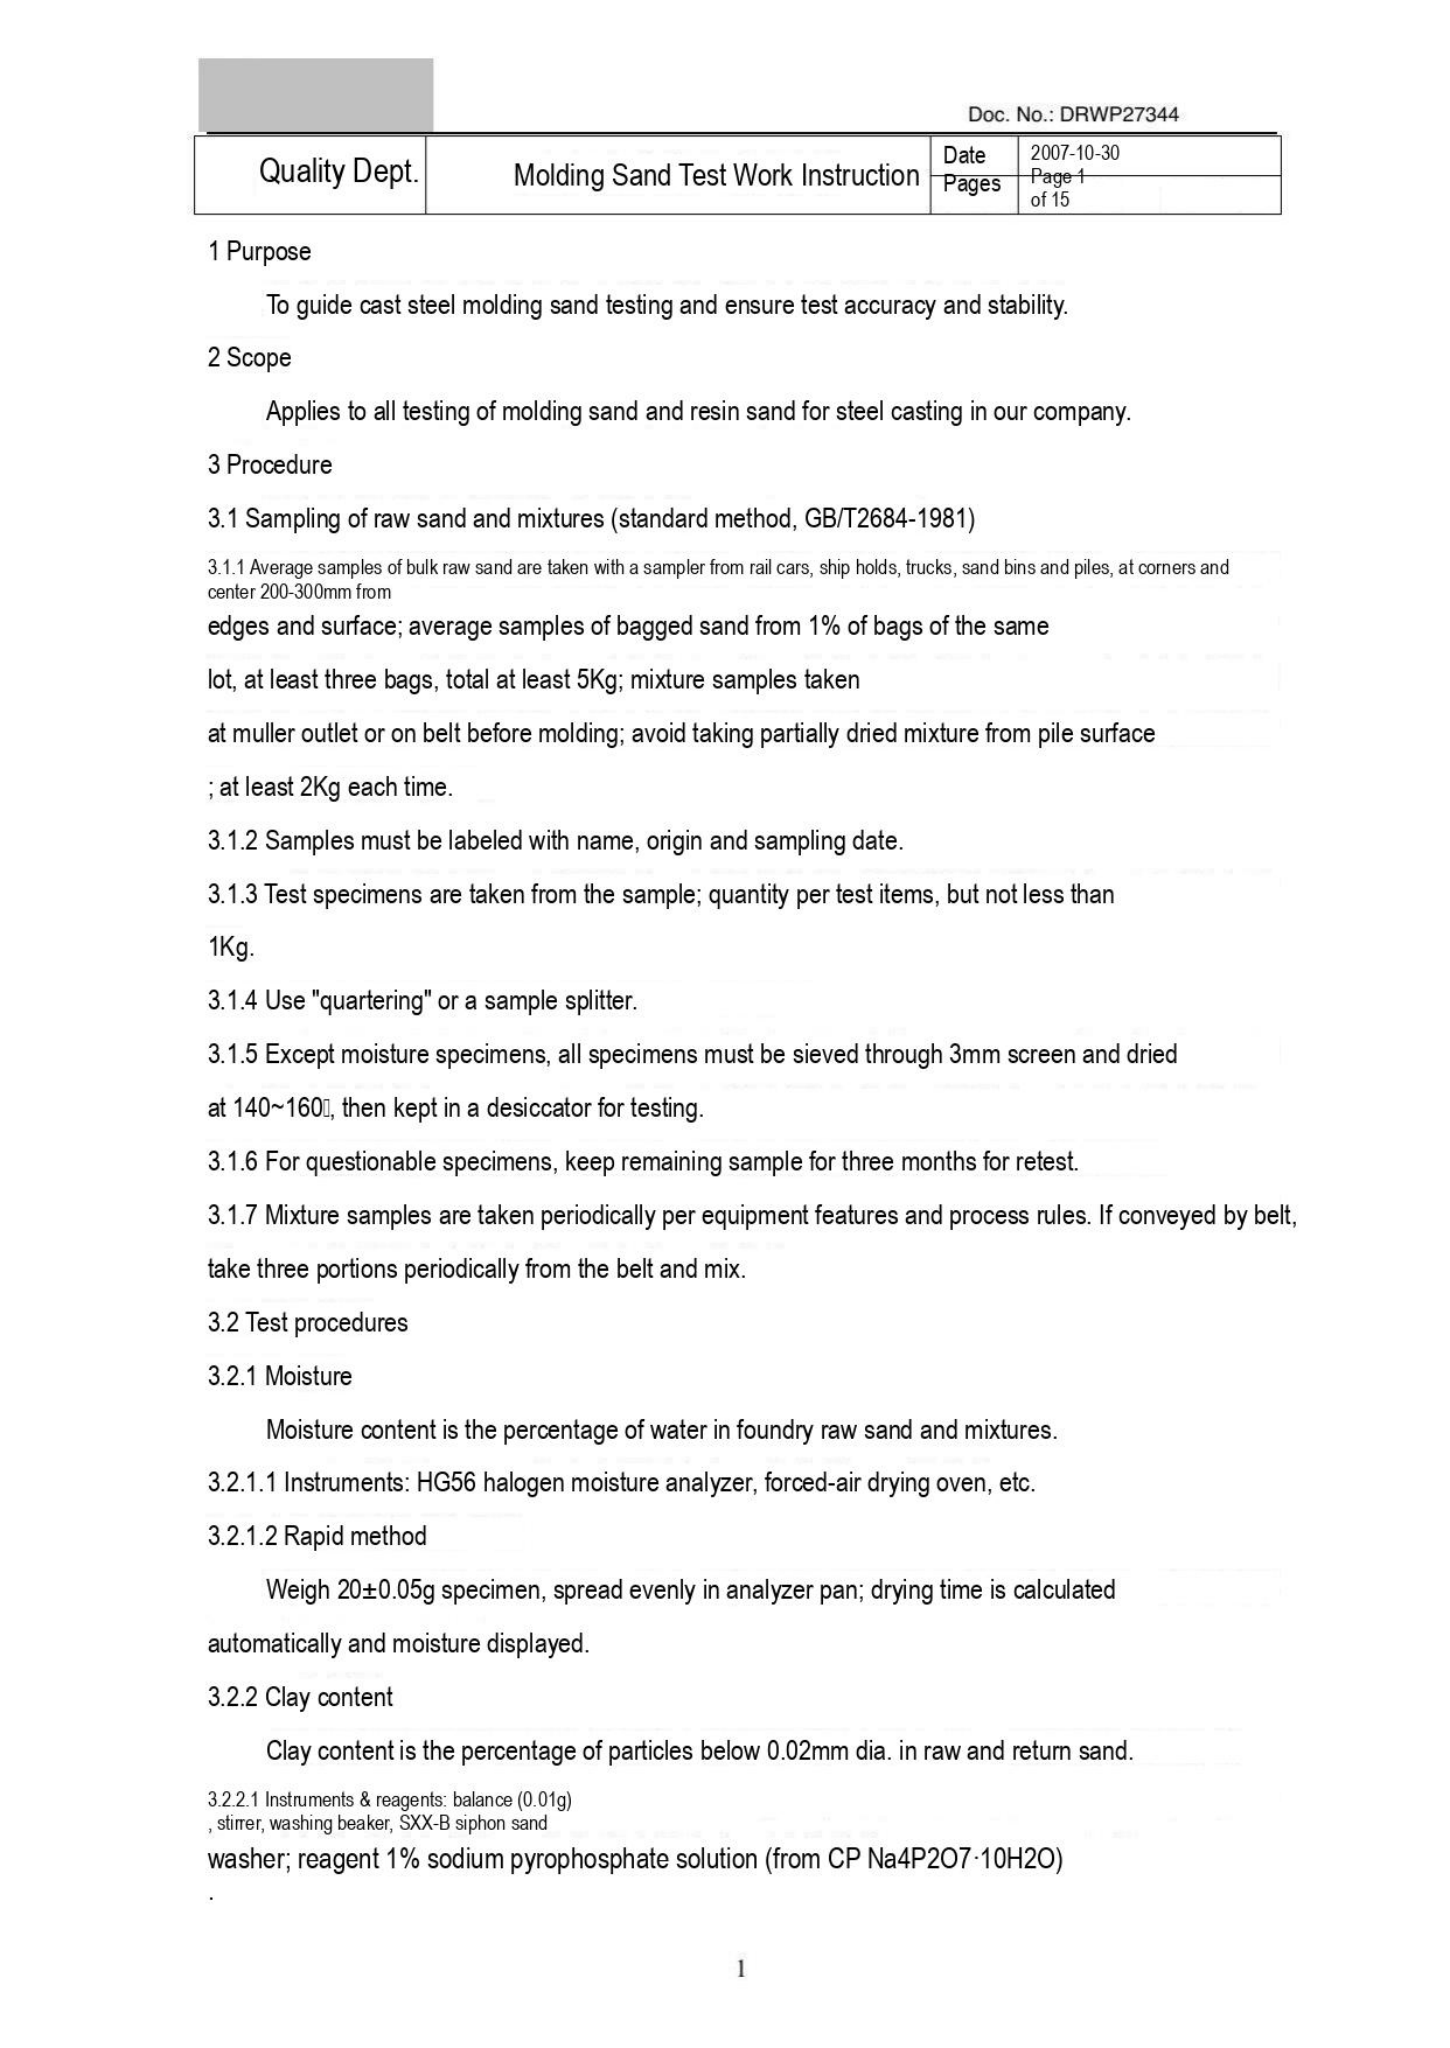Doc. No.: DRWP27344

| Quality Dept. | Molding Sand Test Work Instruction | Date | 2007-10-30 |
|---|---|---|---|
| | | Pages | Page 1 of 15 |

1 Purpose

To guide cast steel molding sand testing and ensure test accuracy and stability.

2 Scope

Applies to all testing of molding sand and resin sand for steel casting in our company.

3 Procedure

3.1 Sampling of raw sand and mixtures (standard method, GB/T2684-1981)

3.1.1 Average samples of bulk raw sand are taken with a sampler from rail cars, ship holds, trucks, sand bins and piles, at corners and center 200-300mm from edges and surface; average samples of bagged sand from 1% of bags of the same lot, at least three bags, total at least 5Kg; mixture samples taken at muller outlet or on belt before molding; avoid taking partially dried mixture from pile surface; at least 2Kg each time.

3.1.2 Samples must be labeled with name, origin and sampling date.

3.1.3 Test specimens are taken from the sample; quantity per test items, but not less than 1Kg.

3.1.4 Use "quartering" or a sample splitter.

3.1.5 Except moisture specimens, all specimens must be sieved through 3mm screen and dried at 140~160, then kept in a desiccator for testing.

3.1.6 For questionable specimens, keep remaining sample for three months for retest.

3.1.7 Mixture samples are taken periodically per equipment features and process rules. If conveyed by belt, take three portions periodically from the belt and mix.

3.2 Test procedures

3.2.1 Moisture

Moisture content is the percentage of water in foundry raw sand and mixtures.

3.2.1.1 Instruments: HG56 halogen moisture analyzer, forced-air drying oven, etc.

3.2.1.2 Rapid method

Weigh 20±0.05g specimen, spread evenly in analyzer pan; drying time is calculated automatically and moisture displayed.

3.2.2 Clay content

Clay content is the percentage of particles below 0.02mm dia. in raw and return sand.

3.2.2.1 Instruments & reagents: balance (0.01g), stirrer, washing beaker, SXX-B siphon sand washer; reagent 1% sodium pyrophosphate solution (from CP Na4P2O7·10H2O).

1
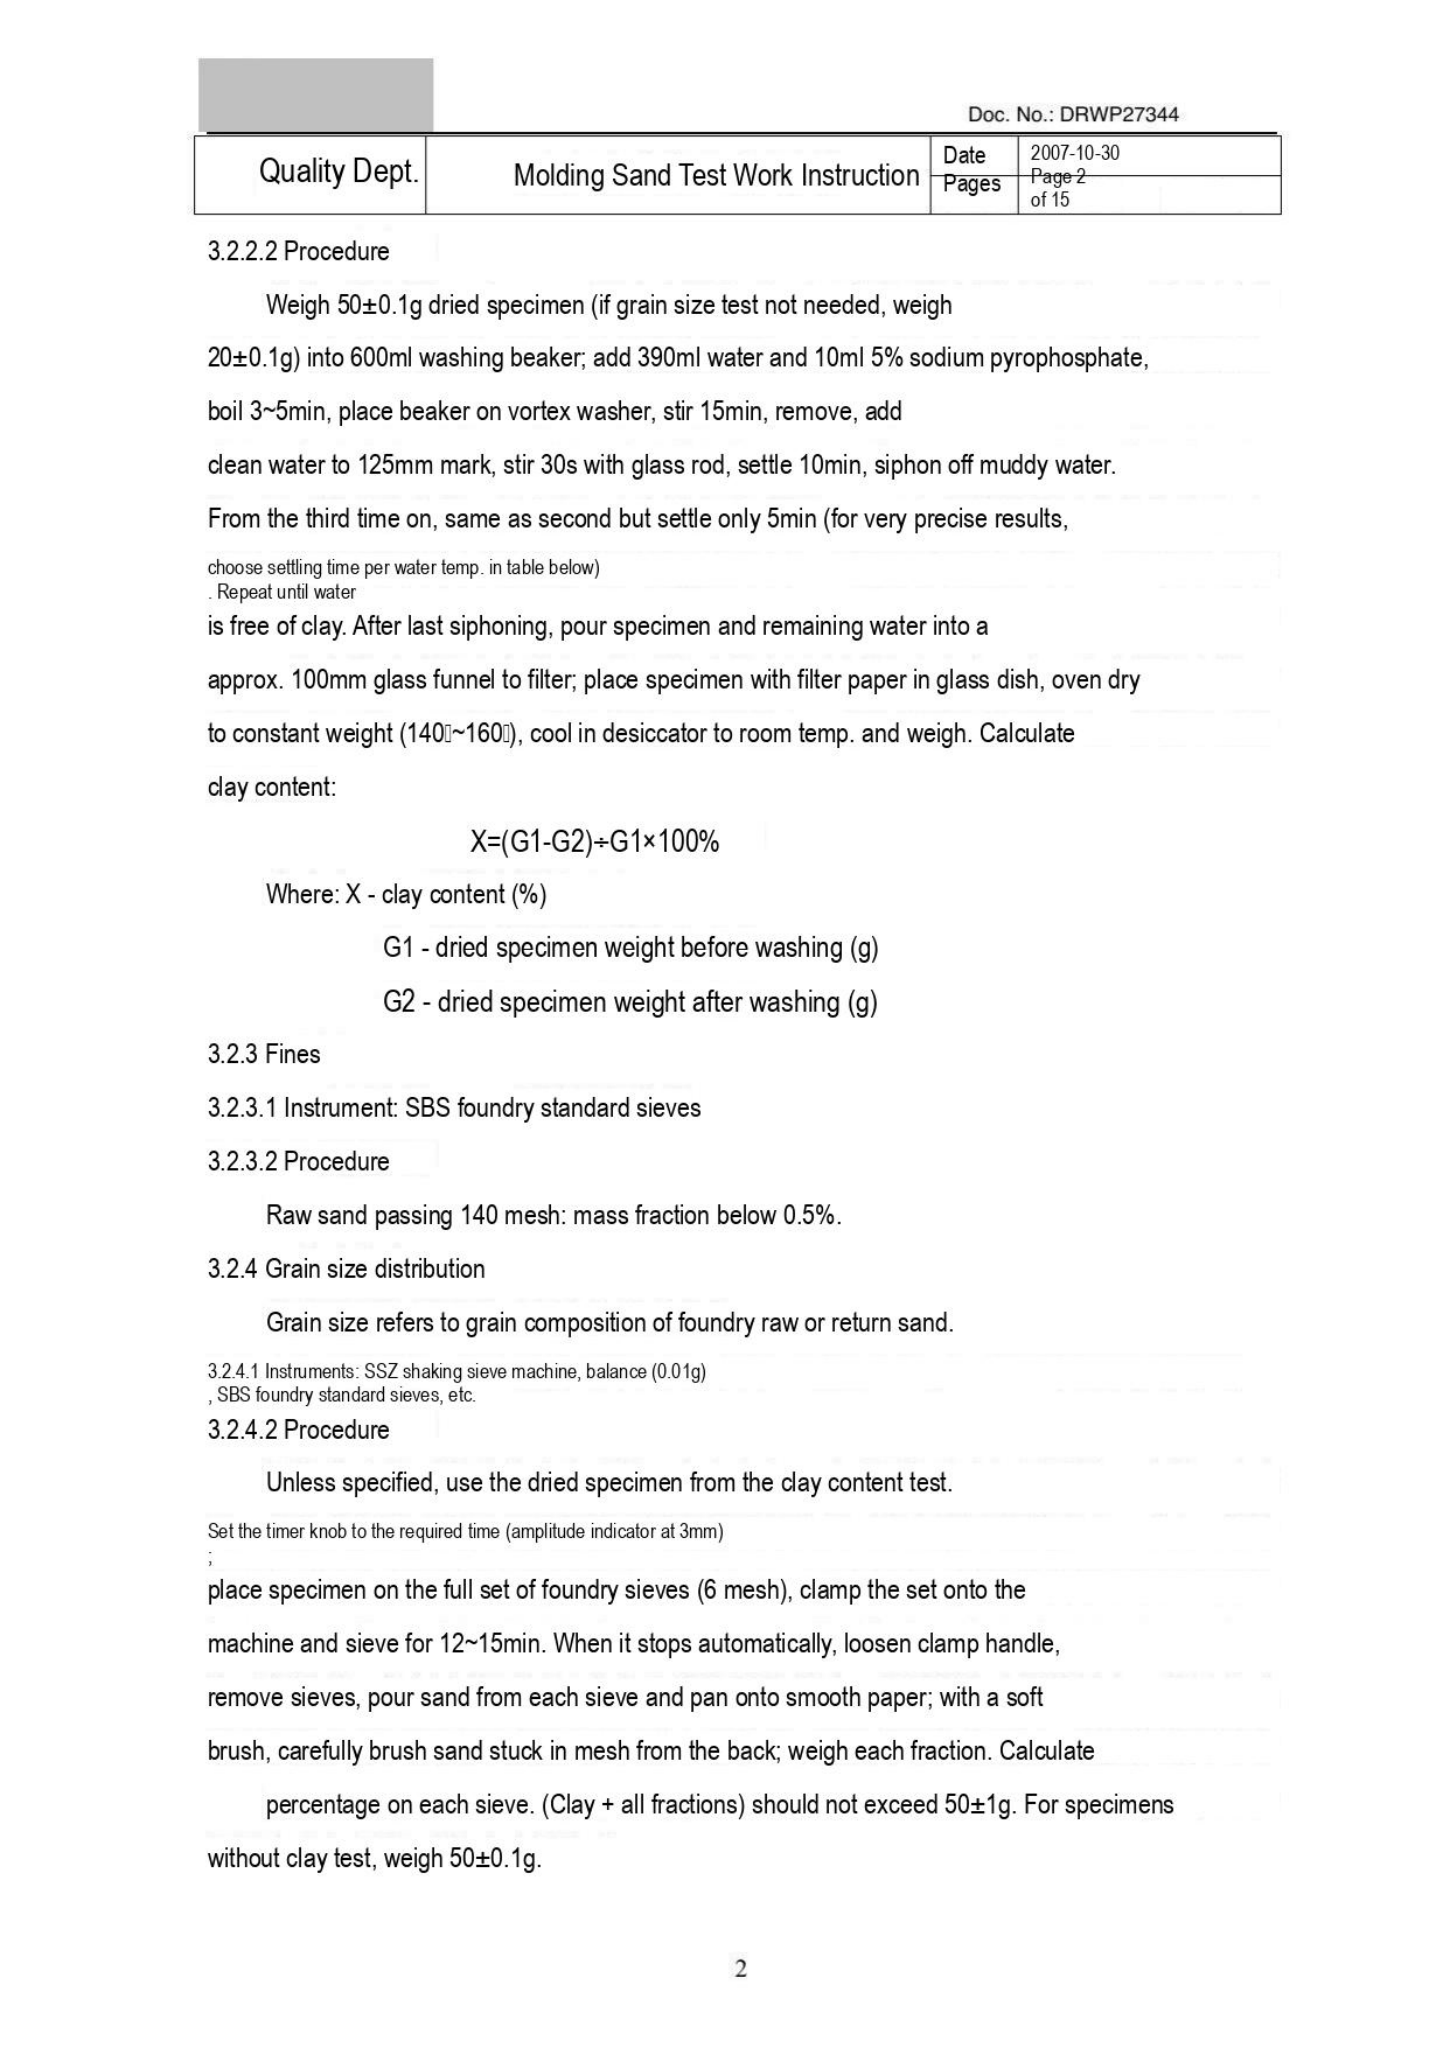Doc. No.: DRWP27344

| Quality Dept. | Molding Sand Test Work Instruction | Date | 2007-10-30 |
|---|---|---|---|
| | | Pages | Page 2 of 15 |

3.2.2.2 Procedure

Weigh 50±0.1g dried specimen (if grain size test not needed, weigh 20±0.1g) into 600ml washing beaker; add 390ml water and 10ml 5% sodium pyrophosphate, boil 3~5min, place beaker on vortex washer, stir 15min, remove, add clean water to 125mm mark, stir 30s with glass rod, settle 10min, siphon off muddy water. From the third time on, same as second but settle only 5min (for very precise results, choose settling time per water temp. in table below). Repeat until water is free of clay. After last siphoning, pour specimen and remaining water into a approx. 100mm glass funnel to filter; place specimen with filter paper in glass dish, oven dry to constant weight (140~160), cool in desiccator to room temp. and weigh. Calculate clay content:

X=(G1-G2)÷G1×100%

Where: X - clay content (%)

G1 - dried specimen weight before washing (g)

G2 - dried specimen weight after washing (g)

3.2.3 Fines

3.2.3.1 Instrument: SBS foundry standard sieves

3.2.3.2 Procedure

Raw sand passing 140 mesh: mass fraction below 0.5%.

3.2.4 Grain size distribution

Grain size refers to grain composition of foundry raw or return sand.

3.2.4.1 Instruments: SSZ shaking sieve machine, balance (0.01g), SBS foundry standard sieves, etc.

3.2.4.2 Procedure

Unless specified, use the dried specimen from the clay content test.

Set the timer knob to the required time (amplitude indicator at 3mm); place specimen on the full set of foundry sieves (6 mesh), clamp the set onto the machine and sieve for 12~15min. When it stops automatically, loosen clamp handle, remove sieves, pour sand from each sieve and pan onto smooth paper; with a soft brush, carefully brush sand stuck in mesh from the back; weigh each fraction. Calculate percentage on each sieve. (Clay + all fractions) should not exceed 50±1g. For specimens without clay test, weigh 50±0.1g.

2
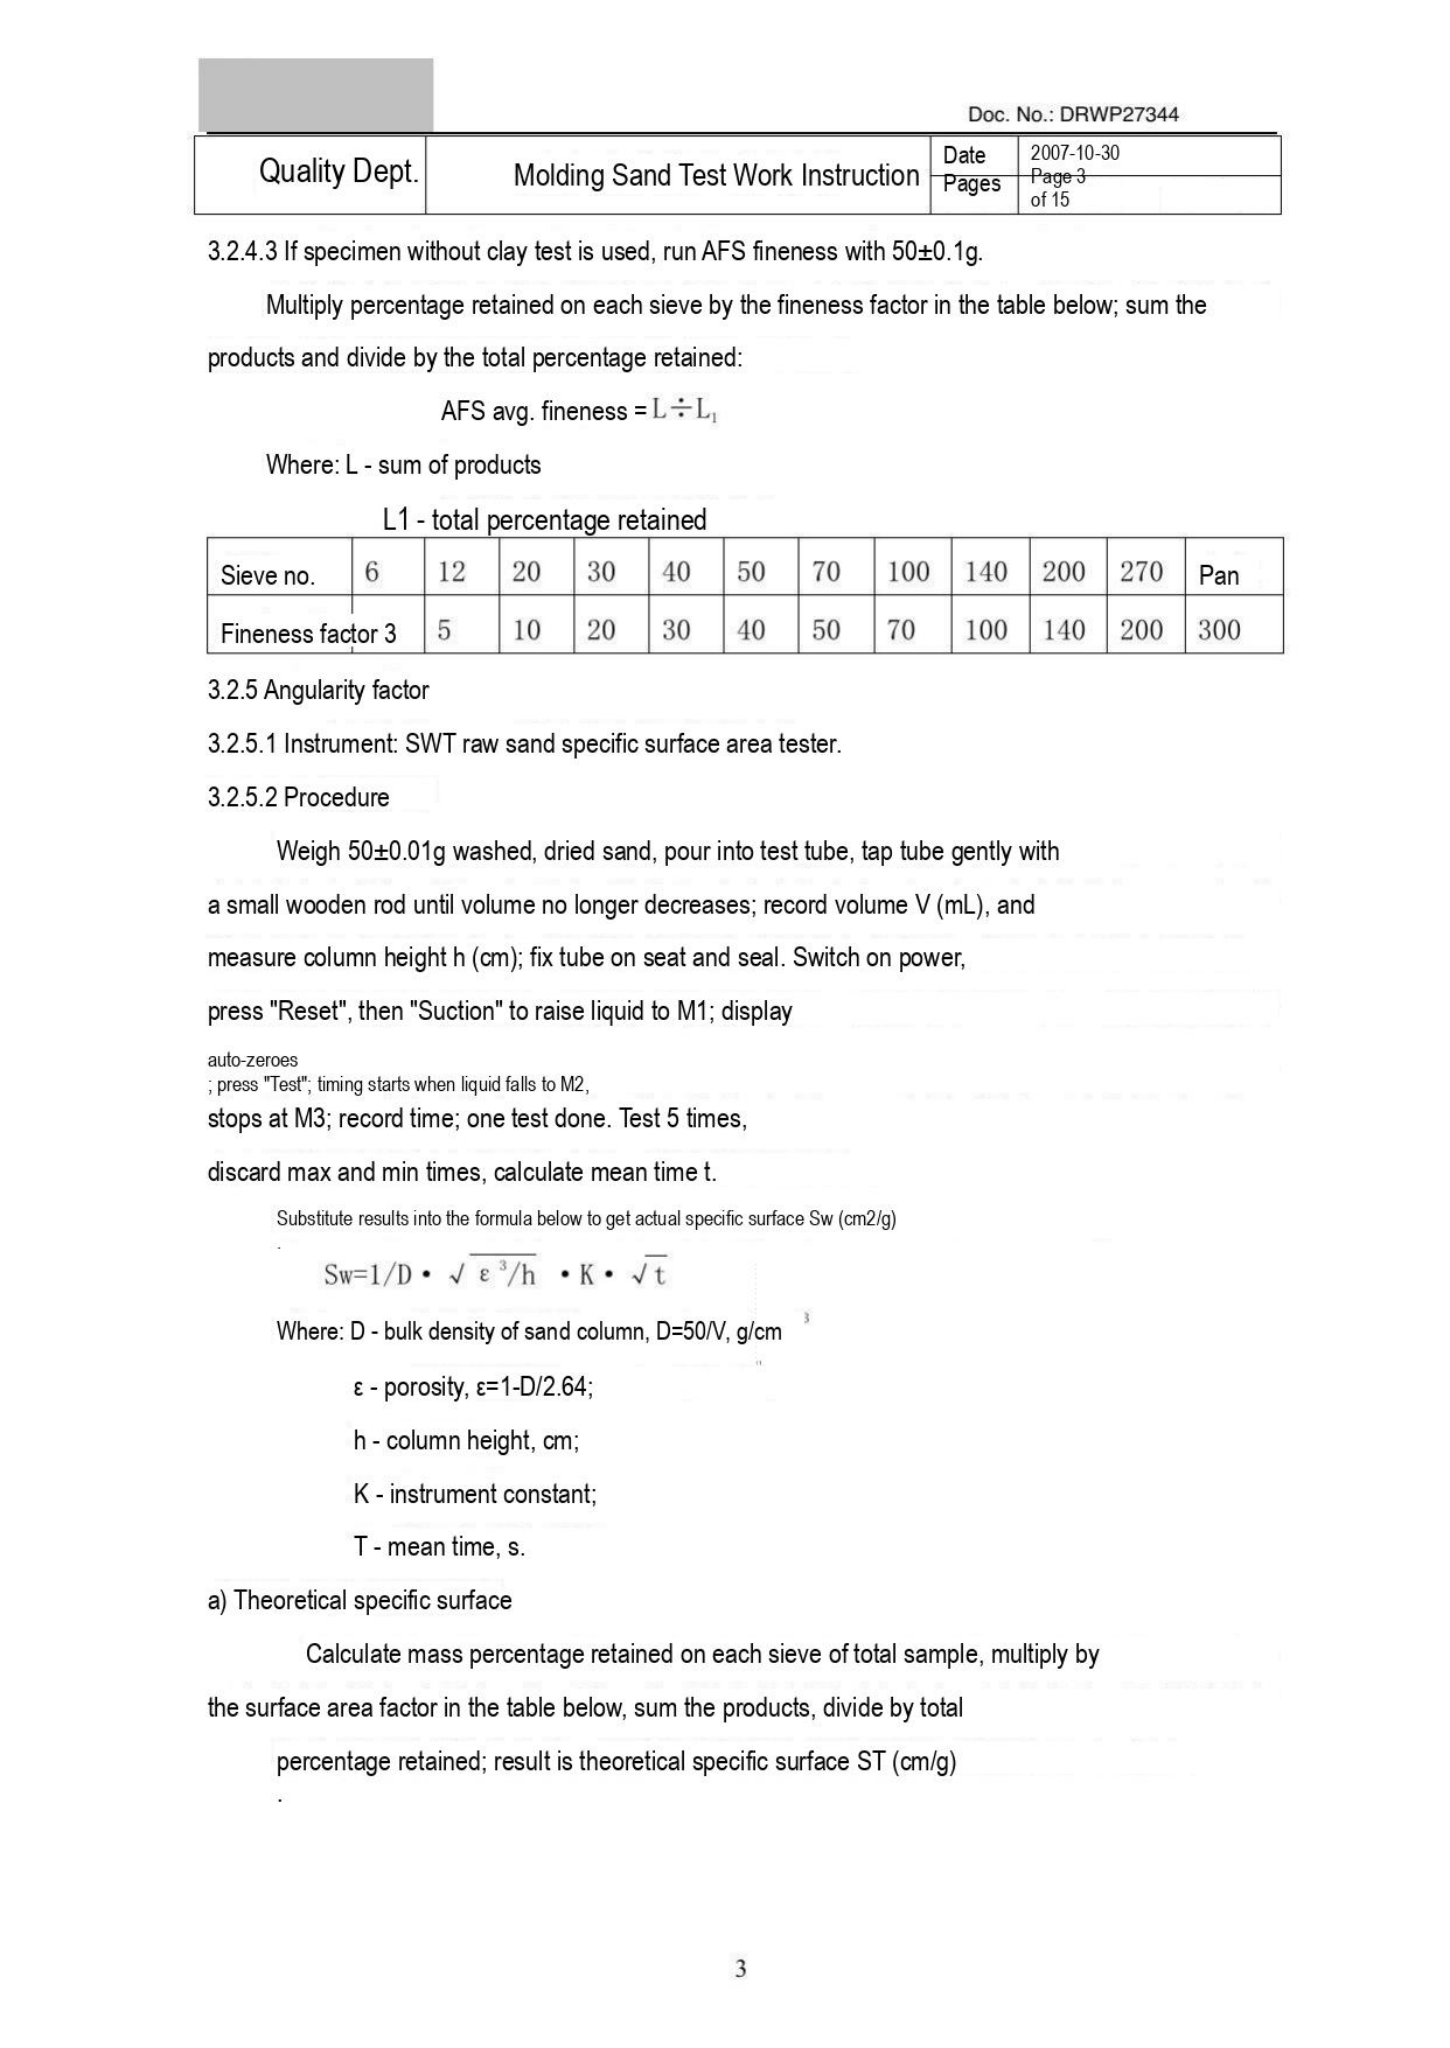Doc. No.: DRWP27344

| Quality Dept. | Molding Sand Test Work Instruction | Date | 2007-10-30 |
|---|---|---|---|
| | | Pages | Page 3 of 15 |

3.2.4.3 If specimen without clay test is used, run AFS fineness with 50±0.1g.

Multiply percentage retained on each sieve by the fineness factor in the table below; sum the products and divide by the total percentage retained:

AFS avg. fineness = L÷L₁

Where: L - sum of products

L1 - total percentage retained

| Sieve no. | 6 | 12 | 20 | 30 | 40 | 50 | 70 | 100 | 140 | 200 | 270 | Pan |
|---|---|---|---|---|---|---|---|---|---|---|---|---|
| Fineness factor | 3 | 5 | 10 | 20 | 30 | 40 | 50 | 70 | 100 | 140 | 200 | 300 |

3.2.5 Angularity factor

3.2.5.1 Instrument: SWT raw sand specific surface area tester.

3.2.5.2 Procedure

Weigh 50±0.01g washed, dried sand, pour into test tube, tap tube gently with a small wooden rod until volume no longer decreases; record volume V (mL), and measure column height h (cm); fix tube on seat and seal. Switch on power, press "Reset", then "Suction" to raise liquid to M1; display auto-zeroes; press "Test"; timing starts when liquid falls to M2, stops at M3; record time; one test done. Test 5 times, discard max and min times, calculate mean time t.

Substitute results into the formula below to get actual specific surface Sw (cm2/g).

Sw=1/D • √ε³/h • K • √t

Where: D - bulk density of sand column, D=50/V, g/cm³

ε - porosity, ε=1-D/2.64;

h - column height, cm;

K - instrument constant;

T - mean time, s.

a) Theoretical specific surface

Calculate mass percentage retained on each sieve of total sample, multiply by the surface area factor in the table below, sum the products, divide by total percentage retained; result is theoretical specific surface ST (cm/g).

3
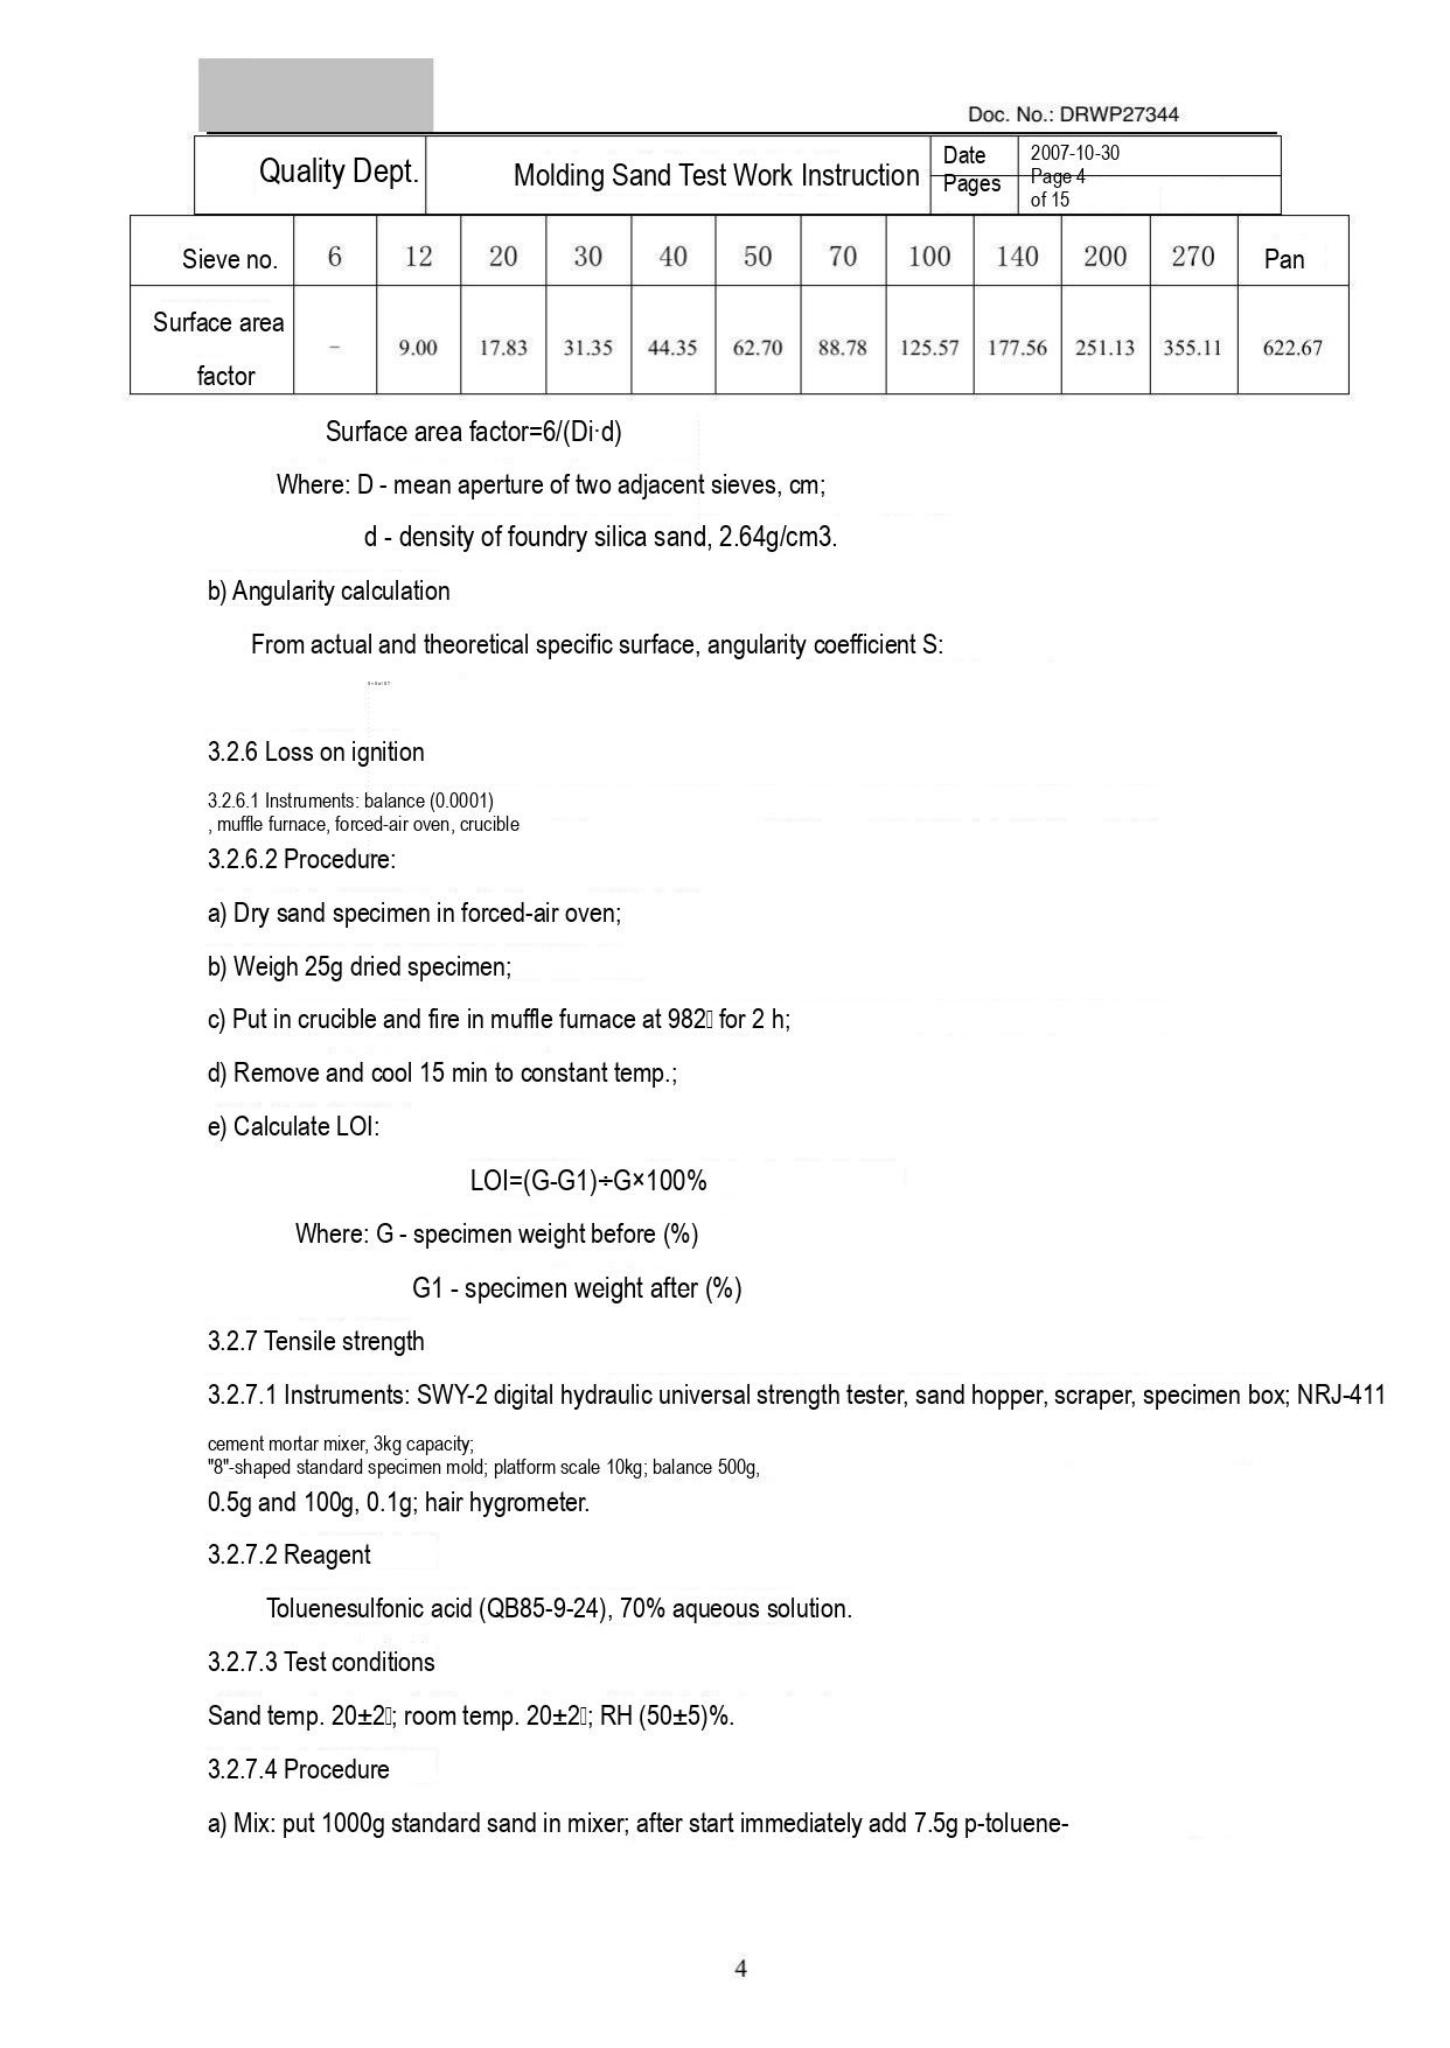Doc. No.: DRWP27344

| Quality Dept. | Molding Sand Test Work Instruction | Date | 2007-10-30 |
|---|---|---|---|
| | | Pages | Page 4 of 15 |

| Sieve no. | 6 | 12 | 20 | 30 | 40 | 50 | 70 | 100 | 140 | 200 | 270 | Pan |
|---|---|---|---|---|---|---|---|---|---|---|---|---|
| Surface area factor | – | 9.00 | 17.83 | 31.35 | 44.35 | 62.70 | 88.78 | 125.57 | 177.56 | 251.13 | 355.11 | 622.67 |

Surface area factor=6/(Di·d)

Where: D - mean aperture of two adjacent sieves, cm;

d - density of foundry silica sand, 2.64g/cm3.

b) Angularity calculation

From actual and theoretical specific surface, angularity coefficient S:

3.2.6 Loss on ignition

3.2.6.1 Instruments: balance (0.0001)
, muffle furnace, forced-air oven, crucible

3.2.6.2 Procedure:

a) Dry sand specimen in forced-air oven;

b) Weigh 25g dried specimen;

c) Put in crucible and fire in muffle furnace at 982 for 2 h;

d) Remove and cool 15 min to constant temp.;

e) Calculate LOI:

LOI=(G-G1)÷G×100%

Where: G - specimen weight before (%)

G1 - specimen weight after (%)

3.2.7 Tensile strength

3.2.7.1 Instruments: SWY-2 digital hydraulic universal strength tester, sand hopper, scraper, specimen box; NRJ-411 cement mortar mixer, 3kg capacity;
"8"-shaped standard specimen mold; platform scale 10kg; balance 500g, 0.5g and 100g, 0.1g; hair hygrometer.

3.2.7.2 Reagent

Toluenesulfonic acid (QB85-9-24), 70% aqueous solution.

3.2.7.3 Test conditions

Sand temp. 20±2; room temp. 20±2; RH (50±5)%.

3.2.7.4 Procedure

a) Mix: put 1000g standard sand in mixer; after start immediately add 7.5g p-toluene-

4
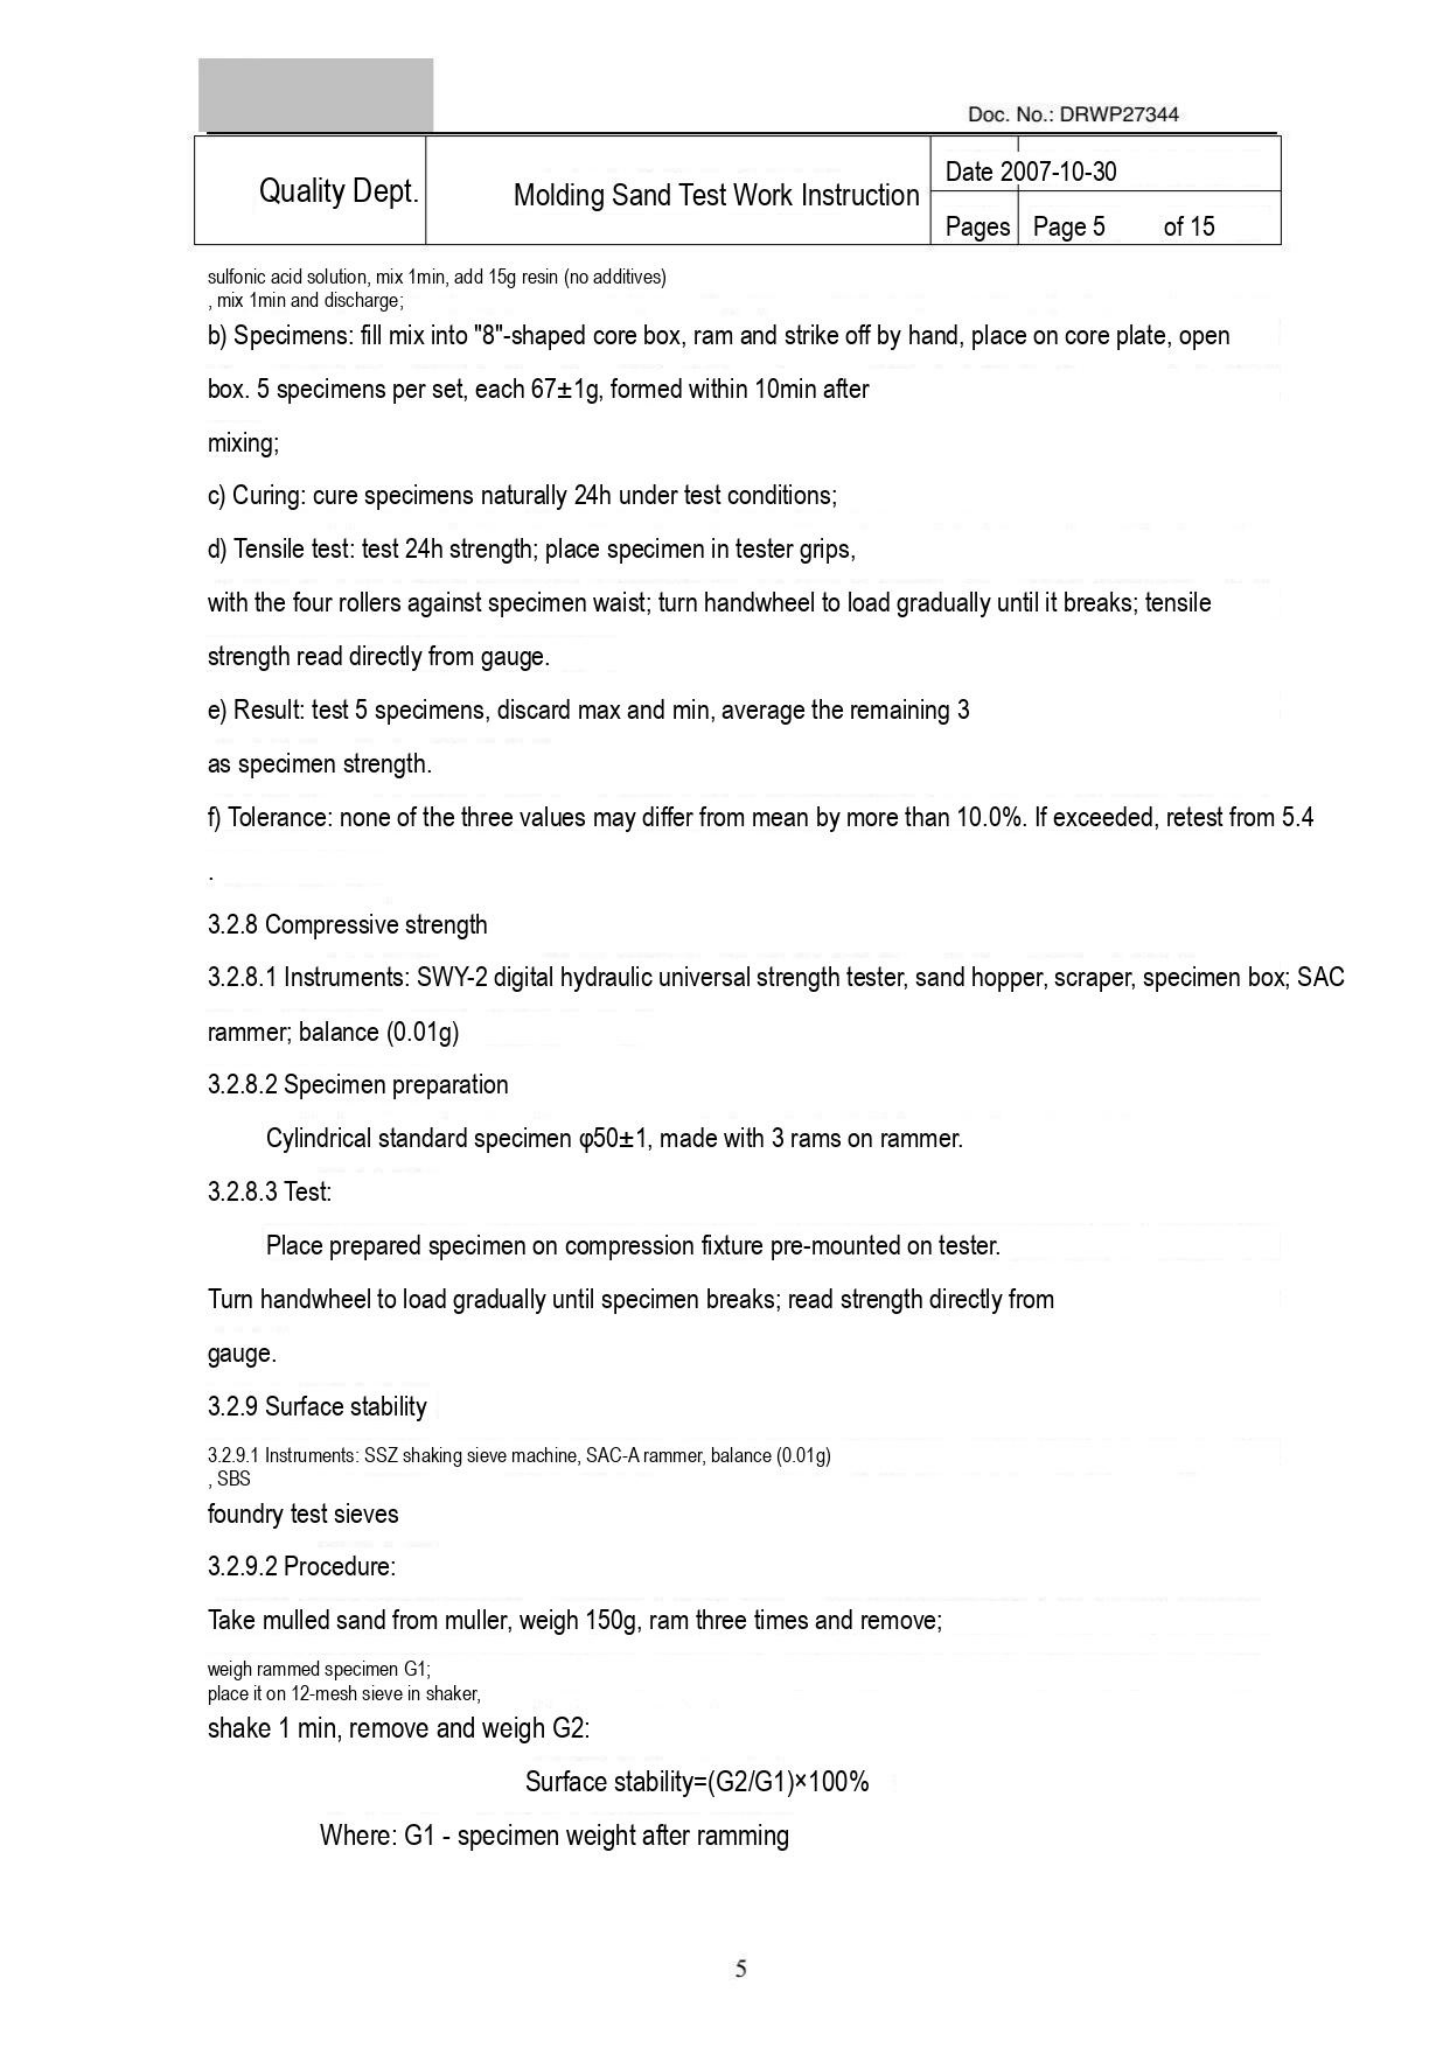Doc. No.: DRWP27344

| Quality Dept. | Molding Sand Test Work Instruction | Date 2007-10-30 | |
|---|---|---|---|
| | | Pages | Page 5 of 15 |

sulfonic acid solution, mix 1min, add 15g resin (no additives)
, mix 1min and discharge;

b) Specimens: fill mix into "8"-shaped core box, ram and strike off by hand, place on core plate, open box. 5 specimens per set, each 67±1g, formed within 10min after mixing;

c) Curing: cure specimens naturally 24h under test conditions;

d) Tensile test: test 24h strength; place specimen in tester grips, with the four rollers against specimen waist; turn handwheel to load gradually until it breaks; tensile strength read directly from gauge.

e) Result: test 5 specimens, discard max and min, average the remaining 3 as specimen strength.

f) Tolerance: none of the three values may differ from mean by more than 10.0%. If exceeded, retest from 5.4
.

3.2.8 Compressive strength

3.2.8.1 Instruments: SWY-2 digital hydraulic universal strength tester, sand hopper, scraper, specimen box; SAC rammer; balance (0.01g)

3.2.8.2 Specimen preparation

Cylindrical standard specimen φ50±1, made with 3 rams on rammer.

3.2.8.3 Test:

Place prepared specimen on compression fixture pre-mounted on tester.

Turn handwheel to load gradually until specimen breaks; read strength directly from gauge.

3.2.9 Surface stability

3.2.9.1 Instruments: SSZ shaking sieve machine, SAC-A rammer, balance (0.01g)
, SBS
foundry test sieves

3.2.9.2 Procedure:

Take mulled sand from muller, weigh 150g, ram three times and remove;

weigh rammed specimen G1;
place it on 12-mesh sieve in shaker,
shake 1 min, remove and weigh G2:

Surface stability=(G2/G1)×100%

Where: G1 - specimen weight after ramming

5
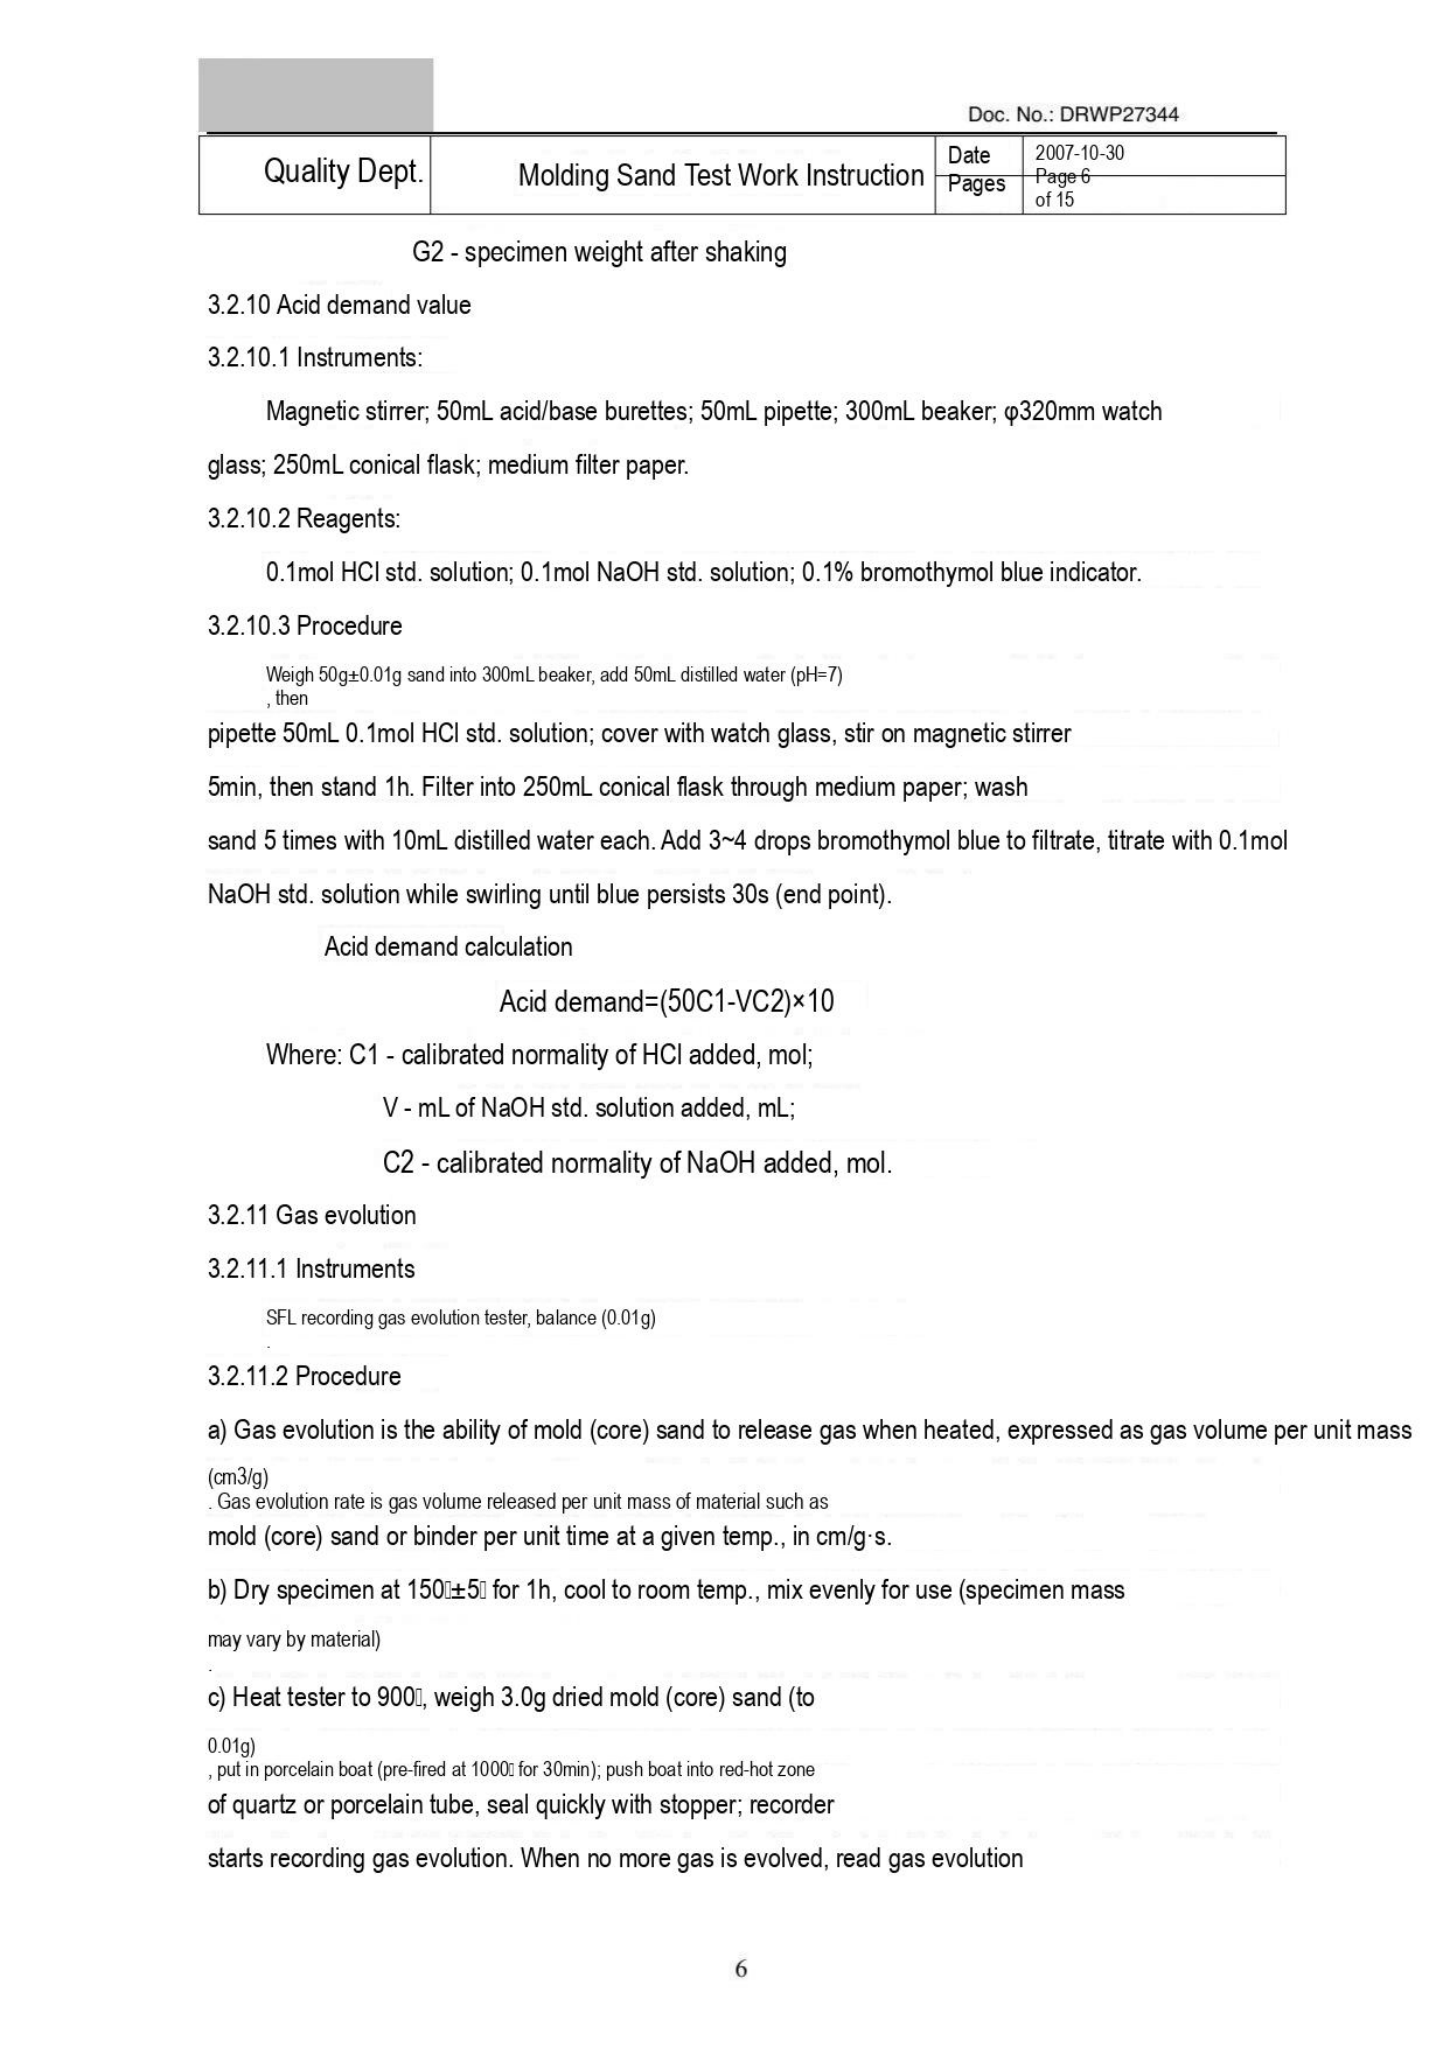Doc. No.: DRWP27344

| Quality Dept. | Molding Sand Test Work Instruction | Date | 2007-10-30 |
|---|---|---|---|
| | | Pages | Page 6 of 15 |

G2 - specimen weight after shaking

3.2.10 Acid demand value

3.2.10.1 Instruments:

Magnetic stirrer; 50mL acid/base burettes; 50mL pipette; 300mL beaker; φ320mm watch glass; 250mL conical flask; medium filter paper.

3.2.10.2 Reagents:

0.1mol HCl std. solution; 0.1mol NaOH std. solution; 0.1% bromothymol blue indicator.

3.2.10.3 Procedure

Weigh 50g±0.01g sand into 300mL beaker, add 50mL distilled water (pH=7), then pipette 50mL 0.1mol HCl std. solution; cover with watch glass, stir on magnetic stirrer 5min, then stand 1h. Filter into 250mL conical flask through medium paper; wash sand 5 times with 10mL distilled water each. Add 3~4 drops bromothymol blue to filtrate, titrate with 0.1mol NaOH std. solution while swirling until blue persists 30s (end point).

Acid demand calculation

Acid demand=(50C1-VC2)×10

Where: C1 - calibrated normality of HCl added, mol;

V - mL of NaOH std. solution added, mL;

C2 - calibrated normality of NaOH added, mol.

3.2.11 Gas evolution

3.2.11.1 Instruments

SFL recording gas evolution tester, balance (0.01g)

3.2.11.2 Procedure

a) Gas evolution is the ability of mold (core) sand to release gas when heated, expressed as gas volume per unit mass (cm3/g). Gas evolution rate is gas volume released per unit mass of material such as mold (core) sand or binder per unit time at a given temp., in cm/g·s.

b) Dry specimen at 150±5 for 1h, cool to room temp., mix evenly for use (specimen mass may vary by material).

c) Heat tester to 900, weigh 3.0g dried mold (core) sand (to 0.01g), put in porcelain boat (pre-fired at 1000 for 30min); push boat into red-hot zone of quartz or porcelain tube, seal quickly with stopper; recorder starts recording gas evolution. When no more gas is evolved, read gas evolution

6